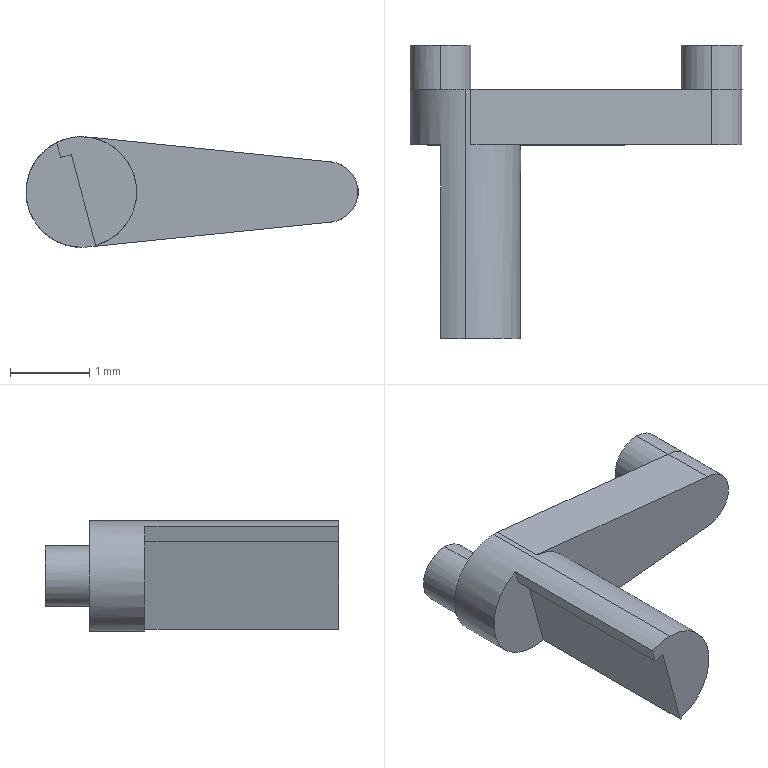Part | SolidWorks | features ICE 2, Extrusion 1, Scale 1 | 1 solid | 19 faces | box 4.201 x 3.71 x 1.4 mm | volume 5.555 mm3 | plane 11 | cylinder 8 | commonest cylinder face diameters 0.77 x3 1.4 x3 0.773 x2
STEP:
#1=CARTESIAN_POINT('',(0.06863,1.198,0.3992));
#2=VERTEX_POINT('',#1);
#3=CARTESIAN_POINT('',(0.06863,1.198,-0.3708));
#4=VERTEX_POINT('',#3);
#5=CARTESIAN_POINT('',(0.06863,1.198,0.0142));
#6=DIRECTION('',(0.,1.,0.));
#7=DIRECTION('',(0.,0.,1.));
#8=AXIS2_PLACEMENT_3D('',#5,#6,#7);
#9=CIRCLE('',#8,0.385);
#10=EDGE_CURVE('',#2,#4,#9,.T.);
#11=ORIENTED_EDGE('',*,*,#10,.F.);
#12=CARTESIAN_POINT('',(0.06863,0.6378,0.3992));
#13=VERTEX_POINT('',#12);
#14=CARTESIAN_POINT('',(0.06863,1.198,0.3992));
#15=DIRECTION('',(0.,-1.,0.));
#16=VECTOR('',#15,1000.);
#17=LINE('',#14,#16);
#18=EDGE_CURVE('',#2,#13,#17,.T.);
#19=ORIENTED_EDGE('',*,*,#18,.T.);
#20=CARTESIAN_POINT('',(0.06863,0.6378,-0.3708));
#21=VERTEX_POINT('',#20);
#22=CARTESIAN_POINT('',(0.06863,0.6378,0.0142));
#23=DIRECTION('',(0.,1.,0.));
#24=DIRECTION('',(0.,0.,1.));
#25=AXIS2_PLACEMENT_3D('',#22,#23,#24);
#26=CIRCLE('',#25,0.385);
#27=EDGE_CURVE('',#13,#21,#26,.T.);
#28=ORIENTED_EDGE('',*,*,#27,.T.);
#29=CARTESIAN_POINT('',(0.06863,1.198,-0.3708));
#30=DIRECTION('',(0.,-1.,0.));
#31=VECTOR('',#30,1000.);
#32=LINE('',#29,#31);
#33=EDGE_CURVE('',#4,#21,#32,.T.);
#34=ORIENTED_EDGE('',*,*,#33,.F.);
#35=EDGE_LOOP('',(#11,#19,#28,#34));
#36=FACE_OUTER_BOUND('',#35,.T.);
#37=CARTESIAN_POINT('',(0.06863,1.198,0.0142));
#38=DIRECTION('',(0.,-1.,0.));
#39=DIRECTION('',(0.,0.,-1.));
#40=AXIS2_PLACEMENT_3D('',#37,#38,#39);
#41=CYLINDRICAL_SURFACE('',#40,0.385);
#42=ADVANCED_FACE('',(#36),#41,.T.);
#43=CARTESIAN_POINT('',(3.499,1.198,0.4006));
#44=VERTEX_POINT('',#43);
#45=CARTESIAN_POINT('',(3.499,1.198,-0.3722));
#46=VERTEX_POINT('',#45);
#47=CARTESIAN_POINT('',(3.499,1.198,0.0142));
#48=DIRECTION('',(0.,1.,0.));
#49=DIRECTION('',(0.,0.,1.));
#50=AXIS2_PLACEMENT_3D('',#47,#48,#49);
#51=CIRCLE('',#50,0.3864);
#52=EDGE_CURVE('',#44,#46,#51,.T.);
#53=ORIENTED_EDGE('',*,*,#52,.F.);
#54=CARTESIAN_POINT('',(3.499,0.6378,0.4006));
#55=VERTEX_POINT('',#54);
#56=CARTESIAN_POINT('',(3.499,1.198,0.4006));
#57=DIRECTION('',(0.,-1.,0.));
#58=VECTOR('',#57,1000.);
#59=LINE('',#56,#58);
#60=EDGE_CURVE('',#44,#55,#59,.T.);
#61=ORIENTED_EDGE('',*,*,#60,.T.);
#62=CARTESIAN_POINT('',(3.499,0.6378,-0.3722));
#63=VERTEX_POINT('',#62);
#64=CARTESIAN_POINT('',(3.499,0.6378,0.0142));
#65=DIRECTION('',(0.,1.,0.));
#66=DIRECTION('',(0.,0.,1.));
#67=AXIS2_PLACEMENT_3D('',#64,#65,#66);
#68=CIRCLE('',#67,0.3864);
#69=EDGE_CURVE('',#55,#63,#68,.T.);
#70=ORIENTED_EDGE('',*,*,#69,.T.);
#71=CARTESIAN_POINT('',(3.499,1.198,-0.3722));
#72=DIRECTION('',(0.,-1.,0.));
#73=VECTOR('',#72,1000.);
#74=LINE('',#71,#73);
#75=EDGE_CURVE('',#46,#63,#74,.T.);
#76=ORIENTED_EDGE('',*,*,#75,.F.);
#77=EDGE_LOOP('',(#53,#61,#70,#76));
#78=FACE_OUTER_BOUND('',#77,.T.);
#79=CARTESIAN_POINT('',(3.499,1.198,0.0142));
#80=DIRECTION('',(0.,-1.,0.));
#81=DIRECTION('',(0.,0.,-1.));
#82=AXIS2_PLACEMENT_3D('',#79,#80,#81);
#83=CYLINDRICAL_SURFACE('',#82,0.3864);
#84=ADVANCED_FACE('',(#78),#83,.T.);
#85=CARTESIAN_POINT('',(0.3836,0.6378,0.7142));
#86=VERTEX_POINT('',#85);
#87=CARTESIAN_POINT('',(0.4549,0.6378,0.7106));
#88=VERTEX_POINT('',#87);
#89=CARTESIAN_POINT('',(0.3836,0.6378,0.0142));
#90=DIRECTION('',(0.,1.,0.));
#91=DIRECTION('',(0.,0.,1.));
#92=AXIS2_PLACEMENT_3D('',#89,#90,#91);
#93=CIRCLE('',#92,0.7);
#94=EDGE_CURVE('',#86,#88,#93,.T.);
#95=ORIENTED_EDGE('',*,*,#94,.F.);
#96=CARTESIAN_POINT('',(0.3836,-2.512,0.7142));
#97=VERTEX_POINT('',#96);
#98=CARTESIAN_POINT('',(0.3836,0.6378,0.7142));
#99=DIRECTION('',(0.,-1.,0.));
#100=VECTOR('',#99,1000.);
#101=LINE('',#98,#100);
#102=EDGE_CURVE('',#86,#97,#101,.T.);
#103=ORIENTED_EDGE('',*,*,#102,.T.);
#104=CARTESIAN_POINT('',(0.5648,-2.512,-0.6619));
#105=VERTEX_POINT('',#104);
#106=CARTESIAN_POINT('',(0.3836,-2.512,0.0142));
#107=DIRECTION('',(0.,-1.,0.));
#108=DIRECTION('',(0.,0.,-1.));
#109=AXIS2_PLACEMENT_3D('',#106,#107,#108);
#110=CIRCLE('',#109,0.7);
#111=EDGE_CURVE('',#105,#97,#110,.T.);
#112=ORIENTED_EDGE('',*,*,#111,.F.);
#113=CARTESIAN_POINT('',(0.5648,-0.06225,-0.6619));
#114=VERTEX_POINT('',#113);
#115=CARTESIAN_POINT('',(0.5648,-2.512,-0.6619));
#116=DIRECTION('',(0.,1.,0.));
#117=VECTOR('',#116,1000.);
#118=LINE('',#115,#117);
#119=EDGE_CURVE('',#105,#114,#118,.T.);
#120=ORIENTED_EDGE('',*,*,#119,.T.);
#121=CARTESIAN_POINT('',(0.4549,-0.06225,0.7106));
#122=VERTEX_POINT('',#121);
#123=CARTESIAN_POINT('',(0.3836,-0.06225,0.0142));
#124=DIRECTION('',(0.,-1.,0.));
#125=DIRECTION('',(0.,0.,-1.));
#126=AXIS2_PLACEMENT_3D('',#123,#124,#125);
#127=CIRCLE('',#126,0.7);
#128=EDGE_CURVE('',#114,#122,#127,.T.);
#129=ORIENTED_EDGE('',*,*,#128,.T.);
#130=CARTESIAN_POINT('',(0.4549,0.6378,0.7106));
#131=DIRECTION('',(0.,-1.,0.));
#132=VECTOR('',#131,1000.);
#133=LINE('',#130,#132);
#134=EDGE_CURVE('',#88,#122,#133,.T.);
#135=ORIENTED_EDGE('',*,*,#134,.F.);
#136=EDGE_LOOP('',(#95,#103,#112,#120,#129,#135));
#137=FACE_OUTER_BOUND('',#136,.T.);
#138=CARTESIAN_POINT('',(0.3836,0.6378,0.0142));
#139=DIRECTION('',(0.,-1.,0.));
#140=DIRECTION('',(0.,0.,-1.));
#141=AXIS2_PLACEMENT_3D('',#138,#139,#140);
#142=CYLINDRICAL_SURFACE('',#141,0.7);
#143=ADVANCED_FACE('',(#137),#142,.T.);
#144=ORIENTED_EDGE('',*,*,#102,.F.);
#145=CARTESIAN_POINT('',(-0.3164,0.6378,0.0142));
#146=VERTEX_POINT('',#145);
#147=CARTESIAN_POINT('',(0.3836,0.6378,0.0142));
#148=DIRECTION('',(0.,1.,0.));
#149=DIRECTION('',(0.,0.,1.));
#150=AXIS2_PLACEMENT_3D('',#147,#148,#149);
#151=CIRCLE('',#150,0.7);
#152=EDGE_CURVE('',#146,#86,#151,.T.);
#153=ORIENTED_EDGE('',*,*,#152,.F.);
#154=CARTESIAN_POINT('',(0.3836,0.6378,-0.6858));
#155=VERTEX_POINT('',#154);
#156=CARTESIAN_POINT('',(0.3836,0.6378,0.0142));
#157=DIRECTION('',(0.,1.,0.));
#158=DIRECTION('',(0.,0.,1.));
#159=AXIS2_PLACEMENT_3D('',#156,#157,#158);
#160=CIRCLE('',#159,0.7);
#161=EDGE_CURVE('',#155,#146,#160,.T.);
#162=ORIENTED_EDGE('',*,*,#161,.F.);
#163=CARTESIAN_POINT('',(0.3836,-0.06225,-0.6858));
#164=VERTEX_POINT('',#163);
#165=CARTESIAN_POINT('',(0.3836,0.6378,-0.6858));
#166=DIRECTION('',(0.,-1.,0.));
#167=VECTOR('',#166,1000.);
#168=LINE('',#165,#167);
#169=EDGE_CURVE('',#155,#164,#168,.T.);
#170=ORIENTED_EDGE('',*,*,#169,.T.);
#171=CARTESIAN_POINT('',(0.07089,-0.06225,0.6405));
#172=VERTEX_POINT('',#171);
#173=CARTESIAN_POINT('',(0.3836,-0.06225,0.0142));
#174=DIRECTION('',(0.,1.,0.));
#175=DIRECTION('',(0.,0.,1.));
#176=AXIS2_PLACEMENT_3D('',#173,#174,#175);
#177=CIRCLE('',#176,0.7);
#178=EDGE_CURVE('',#164,#172,#177,.T.);
#179=ORIENTED_EDGE('',*,*,#178,.T.);
#180=CARTESIAN_POINT('',(0.07089,-2.512,0.6405));
#181=VERTEX_POINT('',#180);
#182=CARTESIAN_POINT('',(0.07089,-2.512,0.6405));
#183=DIRECTION('',(0.,1.,0.));
#184=VECTOR('',#183,1000.);
#185=LINE('',#182,#184);
#186=EDGE_CURVE('',#181,#172,#185,.T.);
#187=ORIENTED_EDGE('',*,*,#186,.F.);
#188=CARTESIAN_POINT('',(0.3836,-2.512,0.0142));
#189=DIRECTION('',(0.,-1.,0.));
#190=DIRECTION('',(0.,0.,-1.));
#191=AXIS2_PLACEMENT_3D('',#188,#189,#190);
#192=CIRCLE('',#191,0.7);
#193=EDGE_CURVE('',#97,#181,#192,.T.);
#194=ORIENTED_EDGE('',*,*,#193,.F.);
#195=EDGE_LOOP('',(#144,#153,#162,#170,#179,#187,#194));
#196=FACE_OUTER_BOUND('',#195,.T.);
#197=CARTESIAN_POINT('',(0.3836,0.6378,0.0142));
#198=DIRECTION('',(0.,-1.,0.));
#199=DIRECTION('',(0.,0.,-1.));
#200=AXIS2_PLACEMENT_3D('',#197,#198,#199);
#201=CYLINDRICAL_SURFACE('',#200,0.7);
#202=ADVANCED_FACE('',(#196),#201,.T.);
#203=ORIENTED_EDGE('',*,*,#128,.F.);
#204=CARTESIAN_POINT('',(0.2568,-0.06225,0.4875));
#205=VERTEX_POINT('',#204);
#206=CARTESIAN_POINT('',(0.5648,-0.06225,-0.6619));
#207=DIRECTION('',(0.2588,0.,-0.9659));
#208=VECTOR('',#207,1000.);
#209=LINE('',#206,#208);
#210=EDGE_CURVE('',#205,#114,#209,.T.);
#211=ORIENTED_EDGE('',*,*,#210,.F.);
#212=CARTESIAN_POINT('',(0.1216,-0.06225,0.4513));
#213=VERTEX_POINT('',#212);
#214=CARTESIAN_POINT('',(0.1216,-0.06225,0.4513));
#215=DIRECTION('',(0.9659,0.,0.2588));
#216=VECTOR('',#215,1000.);
#217=LINE('',#214,#216);
#218=EDGE_CURVE('',#213,#205,#217,.T.);
#219=ORIENTED_EDGE('',*,*,#218,.F.);
#220=CARTESIAN_POINT('',(0.1216,-0.06225,0.4513));
#221=DIRECTION('',(0.2588,0.,-0.9659));
#222=VECTOR('',#221,1000.);
#223=LINE('',#220,#222);
#224=EDGE_CURVE('',#172,#213,#223,.T.);
#225=ORIENTED_EDGE('',*,*,#224,.F.);
#226=ORIENTED_EDGE('',*,*,#178,.F.);
#227=CARTESIAN_POINT('',(0.4549,-0.06225,-0.6822));
#228=VERTEX_POINT('',#227);
#229=CARTESIAN_POINT('',(0.3836,-0.06225,0.0142));
#230=DIRECTION('',(0.,1.,0.));
#231=DIRECTION('',(0.,0.,1.));
#232=AXIS2_PLACEMENT_3D('',#229,#230,#231);
#233=CIRCLE('',#232,0.7);
#234=EDGE_CURVE('',#228,#164,#233,.T.);
#235=ORIENTED_EDGE('',*,*,#234,.F.);
#236=CARTESIAN_POINT('',(3.499,-0.06225,-0.3708));
#237=VERTEX_POINT('',#236);
#238=CARTESIAN_POINT('',(0.4549,-0.06225,-0.6822));
#239=DIRECTION('',(-0.9948,0.,-0.1018));
#240=VECTOR('',#239,1000.);
#241=LINE('',#238,#240);
#242=EDGE_CURVE('',#237,#228,#241,.T.);
#243=ORIENTED_EDGE('',*,*,#242,.F.);
#244=CARTESIAN_POINT('',(3.499,-0.06225,0.3992));
#245=VERTEX_POINT('',#244);
#246=CARTESIAN_POINT('',(3.499,-0.06225,0.0142));
#247=DIRECTION('',(0.,1.,0.));
#248=DIRECTION('',(0.,0.,1.));
#249=AXIS2_PLACEMENT_3D('',#246,#247,#248);
#250=CIRCLE('',#249,0.385);
#251=EDGE_CURVE('',#245,#237,#250,.T.);
#252=ORIENTED_EDGE('',*,*,#251,.F.);
#253=CARTESIAN_POINT('',(0.4549,-0.06225,0.7106));
#254=DIRECTION('',(0.9948,0.,-0.1018));
#255=VECTOR('',#254,1000.);
#256=LINE('',#253,#255);
#257=EDGE_CURVE('',#122,#245,#256,.T.);
#258=ORIENTED_EDGE('',*,*,#257,.F.);
#259=EDGE_LOOP('',(#203,#211,#219,#225,#226,#235,#243,#252,#258));
#260=FACE_OUTER_BOUND('',#259,.T.);
#261=CARTESIAN_POINT('',(0.3836,-0.06225,0.0142));
#262=DIRECTION('',(0.,1.,0.));
#263=DIRECTION('',(0.,0.,1.));
#264=AXIS2_PLACEMENT_3D('',#261,#262,#263);
#265=PLANE('',#264);
#266=ADVANCED_FACE('',(#260),#265,.F.);
#267=ORIENTED_EDGE('',*,*,#169,.F.);
#268=CARTESIAN_POINT('',(0.4549,0.6378,-0.6822));
#269=VERTEX_POINT('',#268);
#270=CARTESIAN_POINT('',(0.3836,0.6378,0.0142));
#271=DIRECTION('',(0.,1.,0.));
#272=DIRECTION('',(0.,0.,1.));
#273=AXIS2_PLACEMENT_3D('',#270,#271,#272);
#274=CIRCLE('',#273,0.7);
#275=EDGE_CURVE('',#269,#155,#274,.T.);
#276=ORIENTED_EDGE('',*,*,#275,.F.);
#277=CARTESIAN_POINT('',(0.4549,0.6378,-0.6822));
#278=DIRECTION('',(0.,-1.,0.));
#279=VECTOR('',#278,1000.);
#280=LINE('',#277,#279);
#281=EDGE_CURVE('',#269,#228,#280,.T.);
#282=ORIENTED_EDGE('',*,*,#281,.T.);
#283=ORIENTED_EDGE('',*,*,#234,.T.);
#284=EDGE_LOOP('',(#267,#276,#282,#283));
#285=FACE_OUTER_BOUND('',#284,.T.);
#286=CARTESIAN_POINT('',(0.3836,0.6378,0.0142));
#287=DIRECTION('',(0.,-1.,0.));
#288=DIRECTION('',(0.,0.,-1.));
#289=AXIS2_PLACEMENT_3D('',#286,#287,#288);
#290=CYLINDRICAL_SURFACE('',#289,0.7);
#291=ADVANCED_FACE('',(#285),#290,.T.);
#292=ORIENTED_EDGE('',*,*,#257,.T.);
#293=CARTESIAN_POINT('',(3.499,0.6378,0.3992));
#294=VERTEX_POINT('',#293);
#295=CARTESIAN_POINT('',(3.499,0.6378,0.3992));
#296=DIRECTION('',(0.,-1.,0.));
#297=VECTOR('',#296,1000.);
#298=LINE('',#295,#297);
#299=EDGE_CURVE('',#294,#245,#298,.T.);
#300=ORIENTED_EDGE('',*,*,#299,.F.);
#301=CARTESIAN_POINT('',(3.486,0.6378,0.4005));
#302=VERTEX_POINT('',#301);
#303=CARTESIAN_POINT('',(0.4549,0.6378,0.7106));
#304=DIRECTION('',(0.9948,0.,-0.1018));
#305=VECTOR('',#304,1000.);
#306=LINE('',#303,#305);
#307=EDGE_CURVE('',#302,#294,#306,.T.);
#308=ORIENTED_EDGE('',*,*,#307,.F.);
#309=CARTESIAN_POINT('',(0.4549,0.6378,0.7106));
#310=DIRECTION('',(0.9948,0.,-0.1018));
#311=VECTOR('',#310,1000.);
#312=LINE('',#309,#311);
#313=EDGE_CURVE('',#88,#302,#312,.T.);
#314=ORIENTED_EDGE('',*,*,#313,.F.);
#315=ORIENTED_EDGE('',*,*,#134,.T.);
#316=EDGE_LOOP('',(#292,#300,#308,#314,#315));
#317=FACE_OUTER_BOUND('',#316,.T.);
#318=CARTESIAN_POINT('',(0.4549,0.6378,0.7106));
#319=DIRECTION('',(-0.1018,0.,-0.9948));
#320=DIRECTION('',(-0.9948,0.,0.1018));
#321=AXIS2_PLACEMENT_3D('',#318,#319,#320);
#322=PLANE('',#321);
#323=ADVANCED_FACE('',(#317),#322,.F.);
#324=ORIENTED_EDGE('',*,*,#251,.T.);
#325=CARTESIAN_POINT('',(3.499,0.6378,-0.3708));
#326=VERTEX_POINT('',#325);
#327=CARTESIAN_POINT('',(3.499,0.6378,-0.3708));
#328=DIRECTION('',(0.,-1.,0.));
#329=VECTOR('',#328,1000.);
#330=LINE('',#327,#329);
#331=EDGE_CURVE('',#326,#237,#330,.T.);
#332=ORIENTED_EDGE('',*,*,#331,.F.);
#333=CARTESIAN_POINT('',(3.499,0.6378,0.0142));
#334=DIRECTION('',(0.,1.,0.));
#335=DIRECTION('',(0.,0.,1.));
#336=AXIS2_PLACEMENT_3D('',#333,#334,#335);
#337=CIRCLE('',#336,0.385);
#338=EDGE_CURVE('',#294,#326,#337,.T.);
#339=ORIENTED_EDGE('',*,*,#338,.F.);
#340=ORIENTED_EDGE('',*,*,#299,.T.);
#341=EDGE_LOOP('',(#324,#332,#339,#340));
#342=FACE_OUTER_BOUND('',#341,.T.);
#343=CARTESIAN_POINT('',(3.499,0.6378,0.0142));
#344=DIRECTION('',(0.,-1.,0.));
#345=DIRECTION('',(0.,0.,-1.));
#346=AXIS2_PLACEMENT_3D('',#343,#344,#345);
#347=CYLINDRICAL_SURFACE('',#346,0.385);
#348=ADVANCED_FACE('',(#342),#347,.T.);
#349=ORIENTED_EDGE('',*,*,#242,.T.);
#350=ORIENTED_EDGE('',*,*,#281,.F.);
#351=CARTESIAN_POINT('',(3.486,0.6378,-0.3721));
#352=VERTEX_POINT('',#351);
#353=CARTESIAN_POINT('',(0.4549,0.6378,-0.6822));
#354=DIRECTION('',(-0.9948,0.,-0.1018));
#355=VECTOR('',#354,1000.);
#356=LINE('',#353,#355);
#357=EDGE_CURVE('',#352,#269,#356,.T.);
#358=ORIENTED_EDGE('',*,*,#357,.F.);
#359=CARTESIAN_POINT('',(0.4549,0.6378,-0.6822));
#360=DIRECTION('',(-0.9948,0.,-0.1018));
#361=VECTOR('',#360,1000.);
#362=LINE('',#359,#361);
#363=EDGE_CURVE('',#326,#352,#362,.T.);
#364=ORIENTED_EDGE('',*,*,#363,.F.);
#365=ORIENTED_EDGE('',*,*,#331,.T.);
#366=EDGE_LOOP('',(#349,#350,#358,#364,#365));
#367=FACE_OUTER_BOUND('',#366,.T.);
#368=CARTESIAN_POINT('',(0.4549,0.6378,-0.6822));
#369=DIRECTION('',(-0.1018,0.,0.9948));
#370=DIRECTION('',(0.9948,0.,0.1018));
#371=AXIS2_PLACEMENT_3D('',#368,#369,#370);
#372=PLANE('',#371);
#373=ADVANCED_FACE('',(#367),#372,.F.);
#374=ORIENTED_EDGE('',*,*,#275,.T.);
#375=ORIENTED_EDGE('',*,*,#161,.T.);
#376=CARTESIAN_POINT('',(0.06863,0.6378,0.0142));
#377=DIRECTION('',(0.,1.,0.));
#378=DIRECTION('',(0.,0.,1.));
#379=AXIS2_PLACEMENT_3D('',#376,#377,#378);
#380=CIRCLE('',#379,0.385);
#381=EDGE_CURVE('',#21,#146,#380,.T.);
#382=ORIENTED_EDGE('',*,*,#381,.F.);
#383=ORIENTED_EDGE('',*,*,#27,.F.);
#384=CARTESIAN_POINT('',(0.06863,0.6378,0.0142));
#385=DIRECTION('',(0.,1.,0.));
#386=DIRECTION('',(0.,0.,1.));
#387=AXIS2_PLACEMENT_3D('',#384,#385,#386);
#388=CIRCLE('',#387,0.385);
#389=EDGE_CURVE('',#146,#13,#388,.T.);
#390=ORIENTED_EDGE('',*,*,#389,.F.);
#391=ORIENTED_EDGE('',*,*,#152,.T.);
#392=ORIENTED_EDGE('',*,*,#94,.T.);
#393=ORIENTED_EDGE('',*,*,#313,.T.);
#394=CARTESIAN_POINT('',(3.499,0.6378,0.0142));
#395=DIRECTION('',(0.,1.,0.));
#396=DIRECTION('',(0.,0.,1.));
#397=AXIS2_PLACEMENT_3D('',#394,#395,#396);
#398=CIRCLE('',#397,0.3864);
#399=EDGE_CURVE('',#352,#302,#398,.T.);
#400=ORIENTED_EDGE('',*,*,#399,.F.);
#401=ORIENTED_EDGE('',*,*,#357,.T.);
#402=EDGE_LOOP('',(#374,#375,#382,#383,#390,#391,#392,#393,#400,#401));
#403=FACE_OUTER_BOUND('',#402,.T.);
#404=CARTESIAN_POINT('',(0.3836,0.6378,0.0142));
#405=DIRECTION('',(0.,1.,0.));
#406=DIRECTION('',(0.,0.,1.));
#407=AXIS2_PLACEMENT_3D('',#404,#405,#406);
#408=PLANE('',#407);
#409=ADVANCED_FACE('',(#403),#408,.T.);
#410=CARTESIAN_POINT('',(3.499,0.6378,0.0142));
#411=DIRECTION('',(0.,1.,0.));
#412=DIRECTION('',(0.,0.,1.));
#413=AXIS2_PLACEMENT_3D('',#410,#411,#412);
#414=CIRCLE('',#413,0.3864);
#415=EDGE_CURVE('',#302,#55,#414,.T.);
#416=ORIENTED_EDGE('',*,*,#415,.F.);
#417=ORIENTED_EDGE('',*,*,#307,.T.);
#418=ORIENTED_EDGE('',*,*,#338,.T.);
#419=ORIENTED_EDGE('',*,*,#363,.T.);
#420=CARTESIAN_POINT('',(3.499,0.6378,0.0142));
#421=DIRECTION('',(0.,1.,0.));
#422=DIRECTION('',(0.,0.,1.));
#423=AXIS2_PLACEMENT_3D('',#420,#421,#422);
#424=CIRCLE('',#423,0.3864);
#425=EDGE_CURVE('',#63,#352,#424,.T.);
#426=ORIENTED_EDGE('',*,*,#425,.F.);
#427=ORIENTED_EDGE('',*,*,#69,.F.);
#428=EDGE_LOOP('',(#416,#417,#418,#419,#426,#427));
#429=FACE_OUTER_BOUND('',#428,.T.);
#430=CARTESIAN_POINT('',(3.499,0.6378,0.0142));
#431=DIRECTION('',(0.,1.,0.));
#432=DIRECTION('',(0.,0.,1.));
#433=AXIS2_PLACEMENT_3D('',#430,#431,#432);
#434=PLANE('',#433);
#435=ADVANCED_FACE('',(#429),#434,.F.);
#436=ORIENTED_EDGE('',*,*,#60,.F.);
#437=CARTESIAN_POINT('',(3.499,1.198,0.0142));
#438=DIRECTION('',(0.,1.,0.));
#439=DIRECTION('',(0.,0.,1.));
#440=AXIS2_PLACEMENT_3D('',#437,#438,#439);
#441=CIRCLE('',#440,0.3864);
#442=EDGE_CURVE('',#46,#44,#441,.T.);
#443=ORIENTED_EDGE('',*,*,#442,.F.);
#444=ORIENTED_EDGE('',*,*,#75,.T.);
#445=ORIENTED_EDGE('',*,*,#425,.T.);
#446=ORIENTED_EDGE('',*,*,#399,.T.);
#447=ORIENTED_EDGE('',*,*,#415,.T.);
#448=EDGE_LOOP('',(#436,#443,#444,#445,#446,#447));
#449=FACE_OUTER_BOUND('',#448,.T.);
#450=CARTESIAN_POINT('',(3.499,1.198,0.0142));
#451=DIRECTION('',(0.,-1.,0.));
#452=DIRECTION('',(0.,0.,-1.));
#453=AXIS2_PLACEMENT_3D('',#450,#451,#452);
#454=CYLINDRICAL_SURFACE('',#453,0.3864);
#455=ADVANCED_FACE('',(#449),#454,.T.);
#456=ORIENTED_EDGE('',*,*,#442,.T.);
#457=ORIENTED_EDGE('',*,*,#52,.T.);
#458=EDGE_LOOP('',(#456,#457));
#459=FACE_OUTER_BOUND('',#458,.T.);
#460=CARTESIAN_POINT('',(3.499,1.198,0.0142));
#461=DIRECTION('',(0.,1.,0.));
#462=DIRECTION('',(0.,0.,1.));
#463=AXIS2_PLACEMENT_3D('',#460,#461,#462);
#464=PLANE('',#463);
#465=ADVANCED_FACE('',(#459),#464,.T.);
#466=ORIENTED_EDGE('',*,*,#18,.F.);
#467=CARTESIAN_POINT('',(0.06863,1.198,0.0142));
#468=DIRECTION('',(0.,1.,0.));
#469=DIRECTION('',(0.,0.,1.));
#470=AXIS2_PLACEMENT_3D('',#467,#468,#469);
#471=CIRCLE('',#470,0.385);
#472=EDGE_CURVE('',#4,#2,#471,.T.);
#473=ORIENTED_EDGE('',*,*,#472,.F.);
#474=ORIENTED_EDGE('',*,*,#33,.T.);
#475=ORIENTED_EDGE('',*,*,#381,.T.);
#476=ORIENTED_EDGE('',*,*,#389,.T.);
#477=EDGE_LOOP('',(#466,#473,#474,#475,#476));
#478=FACE_OUTER_BOUND('',#477,.T.);
#479=CARTESIAN_POINT('',(0.06863,1.198,0.0142));
#480=DIRECTION('',(0.,-1.,0.));
#481=DIRECTION('',(0.,0.,-1.));
#482=AXIS2_PLACEMENT_3D('',#479,#480,#481);
#483=CYLINDRICAL_SURFACE('',#482,0.385);
#484=ADVANCED_FACE('',(#478),#483,.T.);
#485=ORIENTED_EDGE('',*,*,#472,.T.);
#486=ORIENTED_EDGE('',*,*,#10,.T.);
#487=EDGE_LOOP('',(#485,#486));
#488=FACE_OUTER_BOUND('',#487,.T.);
#489=CARTESIAN_POINT('',(0.06863,1.198,0.0142));
#490=DIRECTION('',(0.,1.,0.));
#491=DIRECTION('',(0.,0.,1.));
#492=AXIS2_PLACEMENT_3D('',#489,#490,#491);
#493=PLANE('',#492);
#494=ADVANCED_FACE('',(#488),#493,.T.);
#495=ORIENTED_EDGE('',*,*,#224,.T.);
#496=CARTESIAN_POINT('',(0.1216,-2.512,0.4513));
#497=VERTEX_POINT('',#496);
#498=CARTESIAN_POINT('',(0.1216,-2.512,0.4513));
#499=DIRECTION('',(0.,1.,0.));
#500=VECTOR('',#499,1000.);
#501=LINE('',#498,#500);
#502=EDGE_CURVE('',#497,#213,#501,.T.);
#503=ORIENTED_EDGE('',*,*,#502,.F.);
#504=CARTESIAN_POINT('',(0.1216,-2.512,0.4513));
#505=DIRECTION('',(0.2588,0.,-0.9659));
#506=VECTOR('',#505,1000.);
#507=LINE('',#504,#506);
#508=EDGE_CURVE('',#181,#497,#507,.T.);
#509=ORIENTED_EDGE('',*,*,#508,.F.);
#510=ORIENTED_EDGE('',*,*,#186,.T.);
#511=EDGE_LOOP('',(#495,#503,#509,#510));
#512=FACE_OUTER_BOUND('',#511,.T.);
#513=CARTESIAN_POINT('',(0.1216,-2.512,0.4513));
#514=DIRECTION('',(0.9659,0.,0.2588));
#515=DIRECTION('',(0.2588,0.,-0.9659));
#516=AXIS2_PLACEMENT_3D('',#513,#514,#515);
#517=PLANE('',#516);
#518=ADVANCED_FACE('',(#512),#517,.F.);
#519=ORIENTED_EDGE('',*,*,#218,.T.);
#520=CARTESIAN_POINT('',(0.2568,-2.512,0.4875));
#521=VERTEX_POINT('',#520);
#522=CARTESIAN_POINT('',(0.2568,-2.512,0.4875));
#523=DIRECTION('',(0.,1.,0.));
#524=VECTOR('',#523,1000.);
#525=LINE('',#522,#524);
#526=EDGE_CURVE('',#521,#205,#525,.T.);
#527=ORIENTED_EDGE('',*,*,#526,.F.);
#528=CARTESIAN_POINT('',(0.1216,-2.512,0.4513));
#529=DIRECTION('',(0.9659,0.,0.2588));
#530=VECTOR('',#529,1000.);
#531=LINE('',#528,#530);
#532=EDGE_CURVE('',#497,#521,#531,.T.);
#533=ORIENTED_EDGE('',*,*,#532,.F.);
#534=ORIENTED_EDGE('',*,*,#502,.T.);
#535=EDGE_LOOP('',(#519,#527,#533,#534));
#536=FACE_OUTER_BOUND('',#535,.T.);
#537=CARTESIAN_POINT('',(0.1216,-2.512,0.4513));
#538=DIRECTION('',(-0.2588,0.,0.9659));
#539=DIRECTION('',(0.9659,0.,0.2588));
#540=AXIS2_PLACEMENT_3D('',#537,#538,#539);
#541=PLANE('',#540);
#542=ADVANCED_FACE('',(#536),#541,.F.);
#543=ORIENTED_EDGE('',*,*,#210,.T.);
#544=ORIENTED_EDGE('',*,*,#119,.F.);
#545=CARTESIAN_POINT('',(0.5648,-2.512,-0.6619));
#546=DIRECTION('',(0.2588,0.,-0.9659));
#547=VECTOR('',#546,1000.);
#548=LINE('',#545,#547);
#549=EDGE_CURVE('',#521,#105,#548,.T.);
#550=ORIENTED_EDGE('',*,*,#549,.F.);
#551=ORIENTED_EDGE('',*,*,#526,.T.);
#552=EDGE_LOOP('',(#543,#544,#550,#551));
#553=FACE_OUTER_BOUND('',#552,.T.);
#554=CARTESIAN_POINT('',(0.5648,-2.512,-0.6619));
#555=DIRECTION('',(0.9659,0.,0.2588));
#556=DIRECTION('',(0.2588,0.,-0.9659));
#557=AXIS2_PLACEMENT_3D('',#554,#555,#556);
#558=PLANE('',#557);
#559=ADVANCED_FACE('',(#553),#558,.F.);
#560=ORIENTED_EDGE('',*,*,#111,.T.);
#561=ORIENTED_EDGE('',*,*,#193,.T.);
#562=ORIENTED_EDGE('',*,*,#508,.T.);
#563=ORIENTED_EDGE('',*,*,#532,.T.);
#564=ORIENTED_EDGE('',*,*,#549,.T.);
#565=EDGE_LOOP('',(#560,#561,#562,#563,#564));
#566=FACE_OUTER_BOUND('',#565,.T.);
#567=CARTESIAN_POINT('',(0.3836,-2.512,0.0142));
#568=DIRECTION('',(0.,-1.,0.));
#569=DIRECTION('',(0.,0.,-1.));
#570=AXIS2_PLACEMENT_3D('',#567,#568,#569);
#571=PLANE('',#570);
#572=ADVANCED_FACE('',(#566),#571,.T.);
#573=CLOSED_SHELL('',(#42,#84,#143,#202,#266,#291,#323,#348,#373,#409,#435,#455,#465,#484,#494,#518,#542,#559,#572));
#574=MANIFOLD_SOLID_BREP('',#573);
#575=CARTESIAN_POINT('',(0.,0.,0.));
#576=DIRECTION('',(0.,0.,1.));
#577=DIRECTION('',(1.,0.,0.));
#578=AXIS2_PLACEMENT_3D('',#575,#576,#577);
#579=(LENGTH_UNIT()NAMED_UNIT(*)SI_UNIT(.MILLI.,.METRE.));
#580=UNCERTAINTY_MEASURE_WITH_UNIT(LENGTH_MEASURE(0.00001),#579,'','');
#581=(NAMED_UNIT(*)PLANE_ANGLE_UNIT()SI_UNIT($,.RADIAN.));
#582=(NAMED_UNIT(*)SI_UNIT($,.STERADIAN.)SOLID_ANGLE_UNIT());
#583=(GEOMETRIC_REPRESENTATION_CONTEXT(3)GLOBAL_UNCERTAINTY_ASSIGNED_CONTEXT((#580))GLOBAL_UNIT_ASSIGNED_CONTEXT((#579,#581,#582))REPRESENTATION_CONTEXT('',''));
#584=ADVANCED_BREP_SHAPE_REPRESENTATION('',(#574,#578),#583);